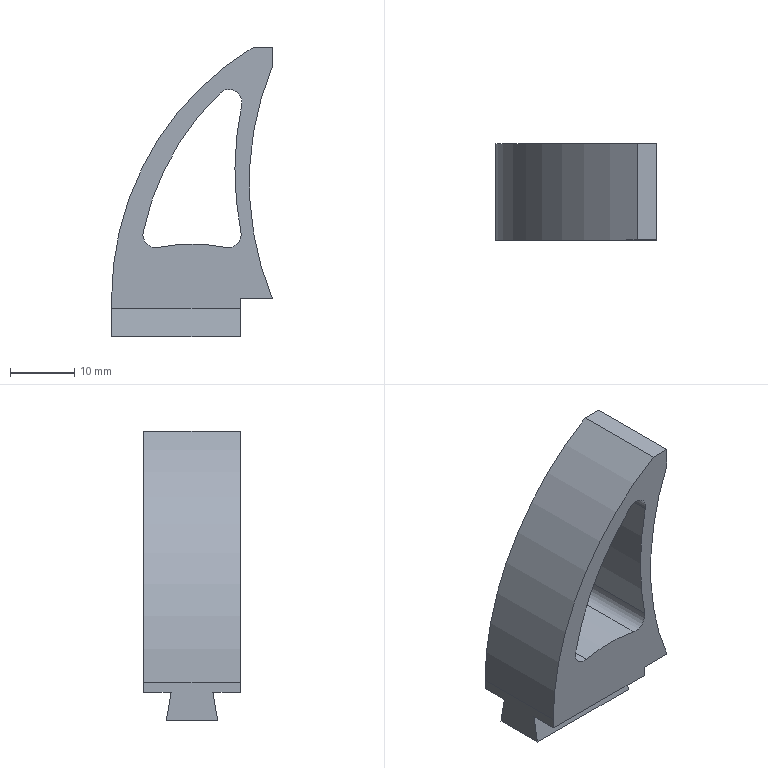Part | NX | features DATUM_CSYS 4, EXTRUDE 3, SKETCH 3, CPROJ 2 | 1 solid | 20 faces | volume 6914 mm3 | plane 12 | cylinder 8 | commonest cylinder face diameters 4 x3 50 x1 84 x1 91.136 x1 94 x1 100 x1